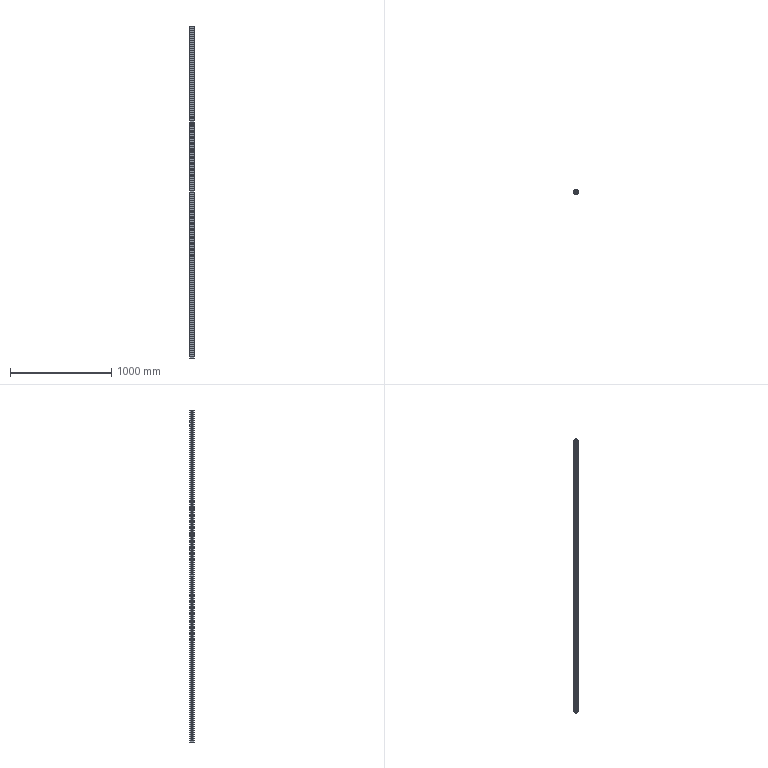Part | SolidWorks | features HoleWzd 5, BaseBody 1, MoveFace 1 | 1 solid | 325 faces | box 40 x 40 x 3280 mm | volume 1938828 mm3 | plane 203 | cylinder 122 | commonest cylinder face diameters 6.8 x48 5 x18 6.6 x16 11 x16 7 x8 1 x6